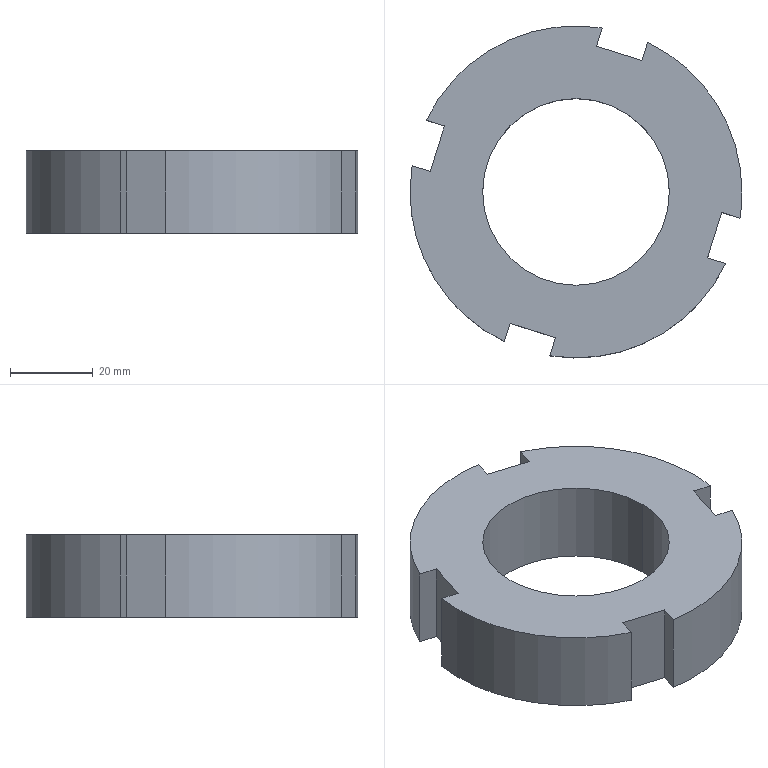Part | SolidWorks | features Extrusion 1 | 1 solid | 21 faces | box 80 x 80 x 20 mm | volume 64249 mm3 | plane 14 | cylinder 7 | commonest cylinder face diameters 80 x5 45 x2
STEP:
#1=CARTESIAN_POINT('',(498.731,234.744,-1569.998));
#2=VERTEX_POINT('',#1);
#3=CARTESIAN_POINT('',(543.731,234.744,-1569.998));
#4=VERTEX_POINT('',#3);
#5=CARTESIAN_POINT('',(521.231,234.744,-1569.998));
#6=DIRECTION('',(0.,0.,1.));
#7=DIRECTION('',(-1.,0.,0.));
#8=AXIS2_PLACEMENT_3D('',#5,#6,#7);
#9=CIRCLE('',#8,22.5);
#10=EDGE_CURVE('',#2,#4,#9,.T.);
#11=ORIENTED_EDGE('',*,*,#10,.F.);
#12=CARTESIAN_POINT('',(498.731,234.744,-1549.998));
#13=VERTEX_POINT('',#12);
#14=CARTESIAN_POINT('',(498.731,234.744,-1569.998));
#15=DIRECTION('',(0.,0.,1.));
#16=VECTOR('',#15,1000.);
#17=LINE('',#14,#16);
#18=EDGE_CURVE('',#2,#13,#17,.T.);
#19=ORIENTED_EDGE('',*,*,#18,.T.);
#20=CARTESIAN_POINT('',(543.731,234.744,-1549.998));
#21=VERTEX_POINT('',#20);
#22=CARTESIAN_POINT('',(521.231,234.744,-1549.998));
#23=DIRECTION('',(0.,0.,1.));
#24=DIRECTION('',(-1.,0.,0.));
#25=AXIS2_PLACEMENT_3D('',#22,#23,#24);
#26=CIRCLE('',#25,22.5);
#27=EDGE_CURVE('',#13,#21,#26,.T.);
#28=ORIENTED_EDGE('',*,*,#27,.T.);
#29=CARTESIAN_POINT('',(543.731,234.744,-1569.998));
#30=DIRECTION('',(0.,0.,1.));
#31=VECTOR('',#30,1000.);
#32=LINE('',#29,#31);
#33=EDGE_CURVE('',#4,#21,#32,.T.);
#34=ORIENTED_EDGE('',*,*,#33,.F.);
#35=EDGE_LOOP('',(#11,#19,#28,#34));
#36=FACE_OUTER_BOUND('',#35,.T.);
#37=CARTESIAN_POINT('',(521.231,234.744,-1569.998));
#38=DIRECTION('',(0.,0.,1.));
#39=DIRECTION('',(1.,0.,0.));
#40=AXIS2_PLACEMENT_3D('',#37,#38,#39);
#41=CYLINDRICAL_SURFACE('',#40,22.5);
#42=ADVANCED_FACE('',(#36),#41,.F.);
#43=CARTESIAN_POINT('',(560.733,228.457,-1569.998));
#44=VERTEX_POINT('',#43);
#45=CARTESIAN_POINT('',(561.231,234.744,-1569.998));
#46=VERTEX_POINT('',#45);
#47=CARTESIAN_POINT('',(521.231,234.744,-1569.998));
#48=DIRECTION('',(0.,0.,1.));
#49=DIRECTION('',(1.,0.,0.));
#50=AXIS2_PLACEMENT_3D('',#47,#48,#49);
#51=CIRCLE('',#50,40.);
#52=EDGE_CURVE('',#44,#46,#51,.T.);
#53=ORIENTED_EDGE('',*,*,#52,.T.);
#54=CARTESIAN_POINT('',(561.231,234.744,-1549.998));
#55=VERTEX_POINT('',#54);
#56=CARTESIAN_POINT('',(561.231,234.744,-1569.998));
#57=DIRECTION('',(0.,0.,1.));
#58=VECTOR('',#57,1000.);
#59=LINE('',#56,#58);
#60=EDGE_CURVE('',#46,#55,#59,.T.);
#61=ORIENTED_EDGE('',*,*,#60,.T.);
#62=CARTESIAN_POINT('',(560.733,228.457,-1549.998));
#63=VERTEX_POINT('',#62);
#64=CARTESIAN_POINT('',(521.231,234.744,-1549.998));
#65=DIRECTION('',(0.,0.,1.));
#66=DIRECTION('',(1.,0.,0.));
#67=AXIS2_PLACEMENT_3D('',#64,#65,#66);
#68=CIRCLE('',#67,40.);
#69=EDGE_CURVE('',#63,#55,#68,.T.);
#70=ORIENTED_EDGE('',*,*,#69,.F.);
#71=CARTESIAN_POINT('',(560.733,228.457,-1569.998));
#72=DIRECTION('',(0.,0.,1.));
#73=VECTOR('',#72,1000.);
#74=LINE('',#71,#73);
#75=EDGE_CURVE('',#44,#63,#74,.T.);
#76=ORIENTED_EDGE('',*,*,#75,.F.);
#77=EDGE_LOOP('',(#53,#61,#70,#76));
#78=FACE_OUTER_BOUND('',#77,.T.);
#79=CARTESIAN_POINT('',(521.231,234.744,-1569.998));
#80=DIRECTION('',(0.,0.,1.));
#81=DIRECTION('',(1.,0.,0.));
#82=AXIS2_PLACEMENT_3D('',#79,#80,#81);
#83=CYLINDRICAL_SURFACE('',#82,40.);
#84=ADVANCED_FACE('',(#78),#83,.T.);
#85=CARTESIAN_POINT('',(537.133,266.448,-1549.998));
#86=VERTEX_POINT('',#85);
#87=CARTESIAN_POINT('',(526.154,269.87,-1549.998));
#88=VERTEX_POINT('',#87);
#89=CARTESIAN_POINT('',(537.133,266.448,-1549.998));
#90=DIRECTION('',(-0.9547,0.2975,0.));
#91=VECTOR('',#90,1000.);
#92=LINE('',#89,#91);
#93=EDGE_CURVE('',#86,#88,#92,.T.);
#94=ORIENTED_EDGE('',*,*,#93,.F.);
#95=CARTESIAN_POINT('',(537.133,266.448,-1569.998));
#96=VERTEX_POINT('',#95);
#97=CARTESIAN_POINT('',(537.133,266.448,-1569.998));
#98=DIRECTION('',(0.,0.,1.));
#99=VECTOR('',#98,1000.);
#100=LINE('',#97,#99);
#101=EDGE_CURVE('',#96,#86,#100,.T.);
#102=ORIENTED_EDGE('',*,*,#101,.F.);
#103=CARTESIAN_POINT('',(526.154,269.87,-1569.998));
#104=VERTEX_POINT('',#103);
#105=CARTESIAN_POINT('',(537.133,266.448,-1569.998));
#106=DIRECTION('',(-0.9547,0.2975,0.));
#107=VECTOR('',#106,1000.);
#108=LINE('',#105,#107);
#109=EDGE_CURVE('',#96,#104,#108,.T.);
#110=ORIENTED_EDGE('',*,*,#109,.T.);
#111=CARTESIAN_POINT('',(526.154,269.87,-1569.998));
#112=DIRECTION('',(0.,0.,1.));
#113=VECTOR('',#112,1000.);
#114=LINE('',#111,#113);
#115=EDGE_CURVE('',#104,#88,#114,.T.);
#116=ORIENTED_EDGE('',*,*,#115,.T.);
#117=EDGE_LOOP('',(#94,#102,#110,#116));
#118=FACE_OUTER_BOUND('',#117,.T.);
#119=CARTESIAN_POINT('',(537.133,266.448,-1569.998));
#120=DIRECTION('',(0.2975,0.9547,0.));
#121=DIRECTION('',(-0.9547,0.2975,0.));
#122=AXIS2_PLACEMENT_3D('',#119,#120,#121);
#123=PLANE('',#122);
#124=ADVANCED_FACE('',(#118),#123,.T.);
#125=CARTESIAN_POINT('',(538.497,270.825,-1549.998));
#126=VERTEX_POINT('',#125);
#127=CARTESIAN_POINT('',(538.497,270.825,-1549.998));
#128=DIRECTION('',(-0.2975,-0.9547,0.));
#129=VECTOR('',#128,1000.);
#130=LINE('',#127,#129);
#131=EDGE_CURVE('',#126,#86,#130,.T.);
#132=ORIENTED_EDGE('',*,*,#131,.F.);
#133=CARTESIAN_POINT('',(538.497,270.825,-1569.998));
#134=VERTEX_POINT('',#133);
#135=CARTESIAN_POINT('',(538.497,270.825,-1569.998));
#136=DIRECTION('',(0.,0.,1.));
#137=VECTOR('',#136,1000.);
#138=LINE('',#135,#137);
#139=EDGE_CURVE('',#134,#126,#138,.T.);
#140=ORIENTED_EDGE('',*,*,#139,.F.);
#141=CARTESIAN_POINT('',(538.497,270.825,-1569.998));
#142=DIRECTION('',(-0.2975,-0.9547,0.));
#143=VECTOR('',#142,1000.);
#144=LINE('',#141,#143);
#145=EDGE_CURVE('',#134,#96,#144,.T.);
#146=ORIENTED_EDGE('',*,*,#145,.T.);
#147=ORIENTED_EDGE('',*,*,#101,.T.);
#148=EDGE_LOOP('',(#132,#140,#146,#147));
#149=FACE_OUTER_BOUND('',#148,.T.);
#150=CARTESIAN_POINT('',(538.497,270.825,-1569.998));
#151=DIRECTION('',(-0.9547,0.2975,0.));
#152=DIRECTION('',(-0.2975,-0.9547,0.));
#153=AXIS2_PLACEMENT_3D('',#150,#151,#152);
#154=PLANE('',#153);
#155=ADVANCED_FACE('',(#149),#154,.T.);
#156=ORIENTED_EDGE('',*,*,#60,.F.);
#157=CARTESIAN_POINT('',(521.231,234.744,-1569.998));
#158=DIRECTION('',(0.,0.,1.));
#159=DIRECTION('',(1.,0.,0.));
#160=AXIS2_PLACEMENT_3D('',#157,#158,#159);
#161=CIRCLE('',#160,40.);
#162=EDGE_CURVE('',#46,#134,#161,.T.);
#163=ORIENTED_EDGE('',*,*,#162,.T.);
#164=ORIENTED_EDGE('',*,*,#139,.T.);
#165=CARTESIAN_POINT('',(521.231,234.744,-1549.998));
#166=DIRECTION('',(0.,0.,1.));
#167=DIRECTION('',(1.,0.,0.));
#168=AXIS2_PLACEMENT_3D('',#165,#166,#167);
#169=CIRCLE('',#168,40.);
#170=EDGE_CURVE('',#55,#126,#169,.T.);
#171=ORIENTED_EDGE('',*,*,#170,.F.);
#172=EDGE_LOOP('',(#156,#163,#164,#171));
#173=FACE_OUTER_BOUND('',#172,.T.);
#174=CARTESIAN_POINT('',(521.231,234.744,-1569.998));
#175=DIRECTION('',(0.,0.,1.));
#176=DIRECTION('',(1.,0.,0.));
#177=AXIS2_PLACEMENT_3D('',#174,#175,#176);
#178=CYLINDRICAL_SURFACE('',#177,40.);
#179=ADVANCED_FACE('',(#173),#178,.T.);
#180=CARTESIAN_POINT('',(556.356,229.821,-1549.998));
#181=VERTEX_POINT('',#180);
#182=CARTESIAN_POINT('',(556.356,229.821,-1549.998));
#183=DIRECTION('',(0.9547,-0.2975,0.));
#184=VECTOR('',#183,1000.);
#185=LINE('',#182,#184);
#186=EDGE_CURVE('',#181,#63,#185,.T.);
#187=ORIENTED_EDGE('',*,*,#186,.F.);
#188=CARTESIAN_POINT('',(556.356,229.821,-1569.998));
#189=VERTEX_POINT('',#188);
#190=CARTESIAN_POINT('',(556.356,229.821,-1569.998));
#191=DIRECTION('',(0.,0.,1.));
#192=VECTOR('',#191,1000.);
#193=LINE('',#190,#192);
#194=EDGE_CURVE('',#189,#181,#193,.T.);
#195=ORIENTED_EDGE('',*,*,#194,.F.);
#196=CARTESIAN_POINT('',(556.356,229.821,-1569.998));
#197=DIRECTION('',(0.9547,-0.2975,0.));
#198=VECTOR('',#197,1000.);
#199=LINE('',#196,#198);
#200=EDGE_CURVE('',#189,#44,#199,.T.);
#201=ORIENTED_EDGE('',*,*,#200,.T.);
#202=ORIENTED_EDGE('',*,*,#75,.T.);
#203=EDGE_LOOP('',(#187,#195,#201,#202));
#204=FACE_OUTER_BOUND('',#203,.T.);
#205=CARTESIAN_POINT('',(556.356,229.821,-1569.998));
#206=DIRECTION('',(-0.2975,-0.9547,0.));
#207=DIRECTION('',(0.9547,-0.2975,0.));
#208=AXIS2_PLACEMENT_3D('',#205,#206,#207);
#209=PLANE('',#208);
#210=ADVANCED_FACE('',(#204),#209,.T.);
#211=CARTESIAN_POINT('',(552.935,218.841,-1549.998));
#212=VERTEX_POINT('',#211);
#213=CARTESIAN_POINT('',(552.935,218.841,-1549.998));
#214=DIRECTION('',(0.2975,0.9547,0.));
#215=VECTOR('',#214,1000.);
#216=LINE('',#213,#215);
#217=EDGE_CURVE('',#212,#181,#216,.T.);
#218=ORIENTED_EDGE('',*,*,#217,.F.);
#219=CARTESIAN_POINT('',(552.935,218.841,-1569.998));
#220=VERTEX_POINT('',#219);
#221=CARTESIAN_POINT('',(552.935,218.841,-1569.998));
#222=DIRECTION('',(0.,0.,1.));
#223=VECTOR('',#222,1000.);
#224=LINE('',#221,#223);
#225=EDGE_CURVE('',#220,#212,#224,.T.);
#226=ORIENTED_EDGE('',*,*,#225,.F.);
#227=CARTESIAN_POINT('',(552.935,218.841,-1569.998));
#228=DIRECTION('',(0.2975,0.9547,0.));
#229=VECTOR('',#228,1000.);
#230=LINE('',#227,#229);
#231=EDGE_CURVE('',#220,#189,#230,.T.);
#232=ORIENTED_EDGE('',*,*,#231,.T.);
#233=ORIENTED_EDGE('',*,*,#194,.T.);
#234=EDGE_LOOP('',(#218,#226,#232,#233));
#235=FACE_OUTER_BOUND('',#234,.T.);
#236=CARTESIAN_POINT('',(552.935,218.841,-1569.998));
#237=DIRECTION('',(0.9547,-0.2975,0.));
#238=DIRECTION('',(0.2975,0.9547,0.));
#239=AXIS2_PLACEMENT_3D('',#236,#237,#238);
#240=PLANE('',#239);
#241=ADVANCED_FACE('',(#235),#240,.T.);
#242=CARTESIAN_POINT('',(557.312,217.477,-1549.998));
#243=VERTEX_POINT('',#242);
#244=CARTESIAN_POINT('',(557.312,217.477,-1549.998));
#245=DIRECTION('',(-0.9547,0.2975,0.));
#246=VECTOR('',#245,1000.);
#247=LINE('',#244,#246);
#248=EDGE_CURVE('',#243,#212,#247,.T.);
#249=ORIENTED_EDGE('',*,*,#248,.F.);
#250=CARTESIAN_POINT('',(557.312,217.477,-1569.998));
#251=VERTEX_POINT('',#250);
#252=CARTESIAN_POINT('',(557.312,217.477,-1569.998));
#253=DIRECTION('',(0.,0.,1.));
#254=VECTOR('',#253,1000.);
#255=LINE('',#252,#254);
#256=EDGE_CURVE('',#251,#243,#255,.T.);
#257=ORIENTED_EDGE('',*,*,#256,.F.);
#258=CARTESIAN_POINT('',(557.312,217.477,-1569.998));
#259=DIRECTION('',(-0.9547,0.2975,0.));
#260=VECTOR('',#259,1000.);
#261=LINE('',#258,#260);
#262=EDGE_CURVE('',#251,#220,#261,.T.);
#263=ORIENTED_EDGE('',*,*,#262,.T.);
#264=ORIENTED_EDGE('',*,*,#225,.T.);
#265=EDGE_LOOP('',(#249,#257,#263,#264));
#266=FACE_OUTER_BOUND('',#265,.T.);
#267=CARTESIAN_POINT('',(557.312,217.477,-1569.998));
#268=DIRECTION('',(0.2975,0.9547,0.));
#269=DIRECTION('',(-0.9547,0.2975,0.));
#270=AXIS2_PLACEMENT_3D('',#267,#268,#269);
#271=PLANE('',#270);
#272=ADVANCED_FACE('',(#266),#271,.T.);
#273=CARTESIAN_POINT('',(514.943,195.241,-1549.998));
#274=VERTEX_POINT('',#273);
#275=CARTESIAN_POINT('',(521.231,234.744,-1549.998));
#276=DIRECTION('',(0.,0.,1.));
#277=DIRECTION('',(1.,0.,0.));
#278=AXIS2_PLACEMENT_3D('',#275,#276,#277);
#279=CIRCLE('',#278,40.);
#280=EDGE_CURVE('',#274,#243,#279,.T.);
#281=ORIENTED_EDGE('',*,*,#280,.F.);
#282=CARTESIAN_POINT('',(514.943,195.241,-1569.998));
#283=VERTEX_POINT('',#282);
#284=CARTESIAN_POINT('',(514.943,195.241,-1569.998));
#285=DIRECTION('',(0.,0.,1.));
#286=VECTOR('',#285,1000.);
#287=LINE('',#284,#286);
#288=EDGE_CURVE('',#283,#274,#287,.T.);
#289=ORIENTED_EDGE('',*,*,#288,.F.);
#290=CARTESIAN_POINT('',(521.231,234.744,-1569.998));
#291=DIRECTION('',(0.,0.,1.));
#292=DIRECTION('',(1.,0.,0.));
#293=AXIS2_PLACEMENT_3D('',#290,#291,#292);
#294=CIRCLE('',#293,40.);
#295=EDGE_CURVE('',#283,#251,#294,.T.);
#296=ORIENTED_EDGE('',*,*,#295,.T.);
#297=ORIENTED_EDGE('',*,*,#256,.T.);
#298=EDGE_LOOP('',(#281,#289,#296,#297));
#299=FACE_OUTER_BOUND('',#298,.T.);
#300=CARTESIAN_POINT('',(521.231,234.744,-1569.998));
#301=DIRECTION('',(0.,0.,1.));
#302=DIRECTION('',(1.,0.,0.));
#303=AXIS2_PLACEMENT_3D('',#300,#301,#302);
#304=CYLINDRICAL_SURFACE('',#303,40.);
#305=ADVANCED_FACE('',(#299),#304,.T.);
#306=CARTESIAN_POINT('',(516.307,199.618,-1549.998));
#307=VERTEX_POINT('',#306);
#308=CARTESIAN_POINT('',(516.307,199.618,-1549.998));
#309=DIRECTION('',(-0.2975,-0.9547,0.));
#310=VECTOR('',#309,1000.);
#311=LINE('',#308,#310);
#312=EDGE_CURVE('',#307,#274,#311,.T.);
#313=ORIENTED_EDGE('',*,*,#312,.F.);
#314=CARTESIAN_POINT('',(516.307,199.618,-1569.998));
#315=VERTEX_POINT('',#314);
#316=CARTESIAN_POINT('',(516.307,199.618,-1569.998));
#317=DIRECTION('',(0.,0.,1.));
#318=VECTOR('',#317,1000.);
#319=LINE('',#316,#318);
#320=EDGE_CURVE('',#315,#307,#319,.T.);
#321=ORIENTED_EDGE('',*,*,#320,.F.);
#322=CARTESIAN_POINT('',(516.307,199.618,-1569.998));
#323=DIRECTION('',(-0.2975,-0.9547,0.));
#324=VECTOR('',#323,1000.);
#325=LINE('',#322,#324);
#326=EDGE_CURVE('',#315,#283,#325,.T.);
#327=ORIENTED_EDGE('',*,*,#326,.T.);
#328=ORIENTED_EDGE('',*,*,#288,.T.);
#329=EDGE_LOOP('',(#313,#321,#327,#328));
#330=FACE_OUTER_BOUND('',#329,.T.);
#331=CARTESIAN_POINT('',(516.307,199.618,-1569.998));
#332=DIRECTION('',(-0.9547,0.2975,0.));
#333=DIRECTION('',(-0.2975,-0.9547,0.));
#334=AXIS2_PLACEMENT_3D('',#331,#332,#333);
#335=PLANE('',#334);
#336=ADVANCED_FACE('',(#330),#335,.T.);
#337=CARTESIAN_POINT('',(505.328,203.04,-1549.998));
#338=VERTEX_POINT('',#337);
#339=CARTESIAN_POINT('',(505.328,203.04,-1549.998));
#340=DIRECTION('',(0.9547,-0.2975,0.));
#341=VECTOR('',#340,1000.);
#342=LINE('',#339,#341);
#343=EDGE_CURVE('',#338,#307,#342,.T.);
#344=ORIENTED_EDGE('',*,*,#343,.F.);
#345=CARTESIAN_POINT('',(505.328,203.04,-1569.998));
#346=VERTEX_POINT('',#345);
#347=CARTESIAN_POINT('',(505.328,203.04,-1569.998));
#348=DIRECTION('',(0.,0.,1.));
#349=VECTOR('',#348,1000.);
#350=LINE('',#347,#349);
#351=EDGE_CURVE('',#346,#338,#350,.T.);
#352=ORIENTED_EDGE('',*,*,#351,.F.);
#353=CARTESIAN_POINT('',(505.328,203.04,-1569.998));
#354=DIRECTION('',(0.9547,-0.2975,0.));
#355=VECTOR('',#354,1000.);
#356=LINE('',#353,#355);
#357=EDGE_CURVE('',#346,#315,#356,.T.);
#358=ORIENTED_EDGE('',*,*,#357,.T.);
#359=ORIENTED_EDGE('',*,*,#320,.T.);
#360=EDGE_LOOP('',(#344,#352,#358,#359));
#361=FACE_OUTER_BOUND('',#360,.T.);
#362=CARTESIAN_POINT('',(505.328,203.04,-1569.998));
#363=DIRECTION('',(-0.2975,-0.9547,0.));
#364=DIRECTION('',(0.9547,-0.2975,0.));
#365=AXIS2_PLACEMENT_3D('',#362,#363,#364);
#366=PLANE('',#365);
#367=ADVANCED_FACE('',(#361),#366,.T.);
#368=CARTESIAN_POINT('',(503.964,198.663,-1549.998));
#369=VERTEX_POINT('',#368);
#370=CARTESIAN_POINT('',(503.964,198.663,-1549.998));
#371=DIRECTION('',(0.2975,0.9547,0.));
#372=VECTOR('',#371,1000.);
#373=LINE('',#370,#372);
#374=EDGE_CURVE('',#369,#338,#373,.T.);
#375=ORIENTED_EDGE('',*,*,#374,.F.);
#376=CARTESIAN_POINT('',(503.964,198.663,-1569.998));
#377=VERTEX_POINT('',#376);
#378=CARTESIAN_POINT('',(503.964,198.663,-1569.998));
#379=DIRECTION('',(0.,0.,1.));
#380=VECTOR('',#379,1000.);
#381=LINE('',#378,#380);
#382=EDGE_CURVE('',#377,#369,#381,.T.);
#383=ORIENTED_EDGE('',*,*,#382,.F.);
#384=CARTESIAN_POINT('',(503.964,198.663,-1569.998));
#385=DIRECTION('',(0.2975,0.9547,0.));
#386=VECTOR('',#385,1000.);
#387=LINE('',#384,#386);
#388=EDGE_CURVE('',#377,#346,#387,.T.);
#389=ORIENTED_EDGE('',*,*,#388,.T.);
#390=ORIENTED_EDGE('',*,*,#351,.T.);
#391=EDGE_LOOP('',(#375,#383,#389,#390));
#392=FACE_OUTER_BOUND('',#391,.T.);
#393=CARTESIAN_POINT('',(503.964,198.663,-1569.998));
#394=DIRECTION('',(0.9547,-0.2975,0.));
#395=DIRECTION('',(0.2975,0.9547,0.));
#396=AXIS2_PLACEMENT_3D('',#393,#394,#395);
#397=PLANE('',#396);
#398=ADVANCED_FACE('',(#392),#397,.T.);
#399=CARTESIAN_POINT('',(481.728,241.031,-1549.998));
#400=VERTEX_POINT('',#399);
#401=CARTESIAN_POINT('',(521.231,234.744,-1549.998));
#402=DIRECTION('',(0.,0.,1.));
#403=DIRECTION('',(1.,0.,0.));
#404=AXIS2_PLACEMENT_3D('',#401,#402,#403);
#405=CIRCLE('',#404,40.);
#406=EDGE_CURVE('',#400,#369,#405,.T.);
#407=ORIENTED_EDGE('',*,*,#406,.F.);
#408=CARTESIAN_POINT('',(481.728,241.031,-1569.998));
#409=VERTEX_POINT('',#408);
#410=CARTESIAN_POINT('',(481.728,241.031,-1569.998));
#411=DIRECTION('',(0.,0.,1.));
#412=VECTOR('',#411,1000.);
#413=LINE('',#410,#412);
#414=EDGE_CURVE('',#409,#400,#413,.T.);
#415=ORIENTED_EDGE('',*,*,#414,.F.);
#416=CARTESIAN_POINT('',(521.231,234.744,-1569.998));
#417=DIRECTION('',(0.,0.,1.));
#418=DIRECTION('',(1.,0.,0.));
#419=AXIS2_PLACEMENT_3D('',#416,#417,#418);
#420=CIRCLE('',#419,40.);
#421=EDGE_CURVE('',#409,#377,#420,.T.);
#422=ORIENTED_EDGE('',*,*,#421,.T.);
#423=ORIENTED_EDGE('',*,*,#382,.T.);
#424=EDGE_LOOP('',(#407,#415,#422,#423));
#425=FACE_OUTER_BOUND('',#424,.T.);
#426=CARTESIAN_POINT('',(521.231,234.744,-1569.998));
#427=DIRECTION('',(0.,0.,1.));
#428=DIRECTION('',(1.,0.,0.));
#429=AXIS2_PLACEMENT_3D('',#426,#427,#428);
#430=CYLINDRICAL_SURFACE('',#429,40.);
#431=ADVANCED_FACE('',(#425),#430,.T.);
#432=CARTESIAN_POINT('',(486.105,239.667,-1549.998));
#433=VERTEX_POINT('',#432);
#434=CARTESIAN_POINT('',(486.105,239.667,-1549.998));
#435=DIRECTION('',(-0.9547,0.2975,0.));
#436=VECTOR('',#435,1000.);
#437=LINE('',#434,#436);
#438=EDGE_CURVE('',#433,#400,#437,.T.);
#439=ORIENTED_EDGE('',*,*,#438,.F.);
#440=CARTESIAN_POINT('',(486.105,239.667,-1569.998));
#441=VERTEX_POINT('',#440);
#442=CARTESIAN_POINT('',(486.105,239.667,-1569.998));
#443=DIRECTION('',(0.,0.,1.));
#444=VECTOR('',#443,1000.);
#445=LINE('',#442,#444);
#446=EDGE_CURVE('',#441,#433,#445,.T.);
#447=ORIENTED_EDGE('',*,*,#446,.F.);
#448=CARTESIAN_POINT('',(486.105,239.667,-1569.998));
#449=DIRECTION('',(-0.9547,0.2975,0.));
#450=VECTOR('',#449,1000.);
#451=LINE('',#448,#450);
#452=EDGE_CURVE('',#441,#409,#451,.T.);
#453=ORIENTED_EDGE('',*,*,#452,.T.);
#454=ORIENTED_EDGE('',*,*,#414,.T.);
#455=EDGE_LOOP('',(#439,#447,#453,#454));
#456=FACE_OUTER_BOUND('',#455,.T.);
#457=CARTESIAN_POINT('',(486.105,239.667,-1569.998));
#458=DIRECTION('',(0.2975,0.9547,0.));
#459=DIRECTION('',(-0.9547,0.2975,0.));
#460=AXIS2_PLACEMENT_3D('',#457,#458,#459);
#461=PLANE('',#460);
#462=ADVANCED_FACE('',(#456),#461,.T.);
#463=CARTESIAN_POINT('',(489.526,250.647,-1549.998));
#464=VERTEX_POINT('',#463);
#465=CARTESIAN_POINT('',(489.526,250.647,-1549.998));
#466=DIRECTION('',(-0.2975,-0.9547,0.));
#467=VECTOR('',#466,1000.);
#468=LINE('',#465,#467);
#469=EDGE_CURVE('',#464,#433,#468,.T.);
#470=ORIENTED_EDGE('',*,*,#469,.F.);
#471=CARTESIAN_POINT('',(489.526,250.647,-1569.998));
#472=VERTEX_POINT('',#471);
#473=CARTESIAN_POINT('',(489.526,250.647,-1569.998));
#474=DIRECTION('',(0.,0.,1.));
#475=VECTOR('',#474,1000.);
#476=LINE('',#473,#475);
#477=EDGE_CURVE('',#472,#464,#476,.T.);
#478=ORIENTED_EDGE('',*,*,#477,.F.);
#479=CARTESIAN_POINT('',(489.526,250.647,-1569.998));
#480=DIRECTION('',(-0.2975,-0.9547,0.));
#481=VECTOR('',#480,1000.);
#482=LINE('',#479,#481);
#483=EDGE_CURVE('',#472,#441,#482,.T.);
#484=ORIENTED_EDGE('',*,*,#483,.T.);
#485=ORIENTED_EDGE('',*,*,#446,.T.);
#486=EDGE_LOOP('',(#470,#478,#484,#485));
#487=FACE_OUTER_BOUND('',#486,.T.);
#488=CARTESIAN_POINT('',(489.526,250.647,-1569.998));
#489=DIRECTION('',(-0.9547,0.2975,0.));
#490=DIRECTION('',(-0.2975,-0.9547,0.));
#491=AXIS2_PLACEMENT_3D('',#488,#489,#490);
#492=PLANE('',#491);
#493=ADVANCED_FACE('',(#487),#492,.T.);
#494=CARTESIAN_POINT('',(485.149,252.011,-1549.998));
#495=VERTEX_POINT('',#494);
#496=CARTESIAN_POINT('',(485.149,252.011,-1549.998));
#497=DIRECTION('',(0.9547,-0.2975,0.));
#498=VECTOR('',#497,1000.);
#499=LINE('',#496,#498);
#500=EDGE_CURVE('',#495,#464,#499,.T.);
#501=ORIENTED_EDGE('',*,*,#500,.F.);
#502=CARTESIAN_POINT('',(485.149,252.011,-1569.998));
#503=VERTEX_POINT('',#502);
#504=CARTESIAN_POINT('',(485.149,252.011,-1569.998));
#505=DIRECTION('',(0.,0.,1.));
#506=VECTOR('',#505,1000.);
#507=LINE('',#504,#506);
#508=EDGE_CURVE('',#503,#495,#507,.T.);
#509=ORIENTED_EDGE('',*,*,#508,.F.);
#510=CARTESIAN_POINT('',(485.149,252.011,-1569.998));
#511=DIRECTION('',(0.9547,-0.2975,0.));
#512=VECTOR('',#511,1000.);
#513=LINE('',#510,#512);
#514=EDGE_CURVE('',#503,#472,#513,.T.);
#515=ORIENTED_EDGE('',*,*,#514,.T.);
#516=ORIENTED_EDGE('',*,*,#477,.T.);
#517=EDGE_LOOP('',(#501,#509,#515,#516));
#518=FACE_OUTER_BOUND('',#517,.T.);
#519=CARTESIAN_POINT('',(485.149,252.011,-1569.998));
#520=DIRECTION('',(-0.2975,-0.9547,0.));
#521=DIRECTION('',(0.9547,-0.2975,0.));
#522=AXIS2_PLACEMENT_3D('',#519,#520,#521);
#523=PLANE('',#522);
#524=ADVANCED_FACE('',(#518),#523,.T.);
#525=CARTESIAN_POINT('',(527.518,274.247,-1549.998));
#526=VERTEX_POINT('',#525);
#527=CARTESIAN_POINT('',(521.231,234.744,-1549.998));
#528=DIRECTION('',(0.,0.,1.));
#529=DIRECTION('',(1.,0.,0.));
#530=AXIS2_PLACEMENT_3D('',#527,#528,#529);
#531=CIRCLE('',#530,40.);
#532=EDGE_CURVE('',#526,#495,#531,.T.);
#533=ORIENTED_EDGE('',*,*,#532,.F.);
#534=CARTESIAN_POINT('',(527.518,274.247,-1569.998));
#535=VERTEX_POINT('',#534);
#536=CARTESIAN_POINT('',(527.518,274.247,-1569.998));
#537=DIRECTION('',(0.,0.,1.));
#538=VECTOR('',#537,1000.);
#539=LINE('',#536,#538);
#540=EDGE_CURVE('',#535,#526,#539,.T.);
#541=ORIENTED_EDGE('',*,*,#540,.F.);
#542=CARTESIAN_POINT('',(521.231,234.744,-1569.998));
#543=DIRECTION('',(0.,0.,1.));
#544=DIRECTION('',(1.,0.,0.));
#545=AXIS2_PLACEMENT_3D('',#542,#543,#544);
#546=CIRCLE('',#545,40.);
#547=EDGE_CURVE('',#535,#503,#546,.T.);
#548=ORIENTED_EDGE('',*,*,#547,.T.);
#549=ORIENTED_EDGE('',*,*,#508,.T.);
#550=EDGE_LOOP('',(#533,#541,#548,#549));
#551=FACE_OUTER_BOUND('',#550,.T.);
#552=CARTESIAN_POINT('',(521.231,234.744,-1569.998));
#553=DIRECTION('',(0.,0.,1.));
#554=DIRECTION('',(1.,0.,0.));
#555=AXIS2_PLACEMENT_3D('',#552,#553,#554);
#556=CYLINDRICAL_SURFACE('',#555,40.);
#557=ADVANCED_FACE('',(#551),#556,.T.);
#558=CARTESIAN_POINT('',(526.154,269.87,-1549.998));
#559=DIRECTION('',(0.2975,0.9547,0.));
#560=VECTOR('',#559,1000.);
#561=LINE('',#558,#560);
#562=EDGE_CURVE('',#88,#526,#561,.T.);
#563=ORIENTED_EDGE('',*,*,#562,.F.);
#564=ORIENTED_EDGE('',*,*,#115,.F.);
#565=CARTESIAN_POINT('',(526.154,269.87,-1569.998));
#566=DIRECTION('',(0.2975,0.9547,0.));
#567=VECTOR('',#566,1000.);
#568=LINE('',#565,#567);
#569=EDGE_CURVE('',#104,#535,#568,.T.);
#570=ORIENTED_EDGE('',*,*,#569,.T.);
#571=ORIENTED_EDGE('',*,*,#540,.T.);
#572=EDGE_LOOP('',(#563,#564,#570,#571));
#573=FACE_OUTER_BOUND('',#572,.T.);
#574=CARTESIAN_POINT('',(526.154,269.87,-1569.998));
#575=DIRECTION('',(0.9547,-0.2975,0.));
#576=DIRECTION('',(0.2975,0.9547,0.));
#577=AXIS2_PLACEMENT_3D('',#574,#575,#576);
#578=PLANE('',#577);
#579=ADVANCED_FACE('',(#573),#578,.T.);
#580=CARTESIAN_POINT('',(521.231,234.744,-1569.998));
#581=DIRECTION('',(0.,0.,1.));
#582=DIRECTION('',(-1.,0.,0.));
#583=AXIS2_PLACEMENT_3D('',#580,#581,#582);
#584=CIRCLE('',#583,22.5);
#585=EDGE_CURVE('',#4,#2,#584,.T.);
#586=ORIENTED_EDGE('',*,*,#585,.T.);
#587=ORIENTED_EDGE('',*,*,#10,.T.);
#588=EDGE_LOOP('',(#586,#587));
#589=FACE_BOUND('',#588,.T.);
#590=ORIENTED_EDGE('',*,*,#109,.F.);
#591=ORIENTED_EDGE('',*,*,#145,.F.);
#592=ORIENTED_EDGE('',*,*,#162,.F.);
#593=ORIENTED_EDGE('',*,*,#52,.F.);
#594=ORIENTED_EDGE('',*,*,#200,.F.);
#595=ORIENTED_EDGE('',*,*,#231,.F.);
#596=ORIENTED_EDGE('',*,*,#262,.F.);
#597=ORIENTED_EDGE('',*,*,#295,.F.);
#598=ORIENTED_EDGE('',*,*,#326,.F.);
#599=ORIENTED_EDGE('',*,*,#357,.F.);
#600=ORIENTED_EDGE('',*,*,#388,.F.);
#601=ORIENTED_EDGE('',*,*,#421,.F.);
#602=ORIENTED_EDGE('',*,*,#452,.F.);
#603=ORIENTED_EDGE('',*,*,#483,.F.);
#604=ORIENTED_EDGE('',*,*,#514,.F.);
#605=ORIENTED_EDGE('',*,*,#547,.F.);
#606=ORIENTED_EDGE('',*,*,#569,.F.);
#607=EDGE_LOOP('',(#590,#591,#592,#593,#594,#595,#596,#597,#598,#599,#600,#601,#602,#603,#604,#605,#606));
#608=FACE_OUTER_BOUND('',#607,.T.);
#609=CARTESIAN_POINT('',(521.231,234.744,-1569.998));
#610=DIRECTION('',(0.,0.,1.));
#611=DIRECTION('',(1.,0.,0.));
#612=AXIS2_PLACEMENT_3D('',#609,#610,#611);
#613=PLANE('',#612);
#614=ADVANCED_FACE('',(#589,#608),#613,.F.);
#615=CARTESIAN_POINT('',(521.231,234.744,-1549.998));
#616=DIRECTION('',(0.,0.,1.));
#617=DIRECTION('',(-1.,0.,0.));
#618=AXIS2_PLACEMENT_3D('',#615,#616,#617);
#619=CIRCLE('',#618,22.5);
#620=EDGE_CURVE('',#21,#13,#619,.T.);
#621=ORIENTED_EDGE('',*,*,#620,.F.);
#622=ORIENTED_EDGE('',*,*,#27,.F.);
#623=EDGE_LOOP('',(#621,#622));
#624=FACE_BOUND('',#623,.T.);
#625=ORIENTED_EDGE('',*,*,#93,.T.);
#626=ORIENTED_EDGE('',*,*,#562,.T.);
#627=ORIENTED_EDGE('',*,*,#532,.T.);
#628=ORIENTED_EDGE('',*,*,#500,.T.);
#629=ORIENTED_EDGE('',*,*,#469,.T.);
#630=ORIENTED_EDGE('',*,*,#438,.T.);
#631=ORIENTED_EDGE('',*,*,#406,.T.);
#632=ORIENTED_EDGE('',*,*,#374,.T.);
#633=ORIENTED_EDGE('',*,*,#343,.T.);
#634=ORIENTED_EDGE('',*,*,#312,.T.);
#635=ORIENTED_EDGE('',*,*,#280,.T.);
#636=ORIENTED_EDGE('',*,*,#248,.T.);
#637=ORIENTED_EDGE('',*,*,#217,.T.);
#638=ORIENTED_EDGE('',*,*,#186,.T.);
#639=ORIENTED_EDGE('',*,*,#69,.T.);
#640=ORIENTED_EDGE('',*,*,#170,.T.);
#641=ORIENTED_EDGE('',*,*,#131,.T.);
#642=EDGE_LOOP('',(#625,#626,#627,#628,#629,#630,#631,#632,#633,#634,#635,#636,#637,#638,#639,#640,#641));
#643=FACE_OUTER_BOUND('',#642,.T.);
#644=CARTESIAN_POINT('',(521.231,234.744,-1549.998));
#645=DIRECTION('',(0.,0.,1.));
#646=DIRECTION('',(1.,0.,0.));
#647=AXIS2_PLACEMENT_3D('',#644,#645,#646);
#648=PLANE('',#647);
#649=ADVANCED_FACE('',(#624,#643),#648,.T.);
#650=ORIENTED_EDGE('',*,*,#18,.F.);
#651=ORIENTED_EDGE('',*,*,#585,.F.);
#652=ORIENTED_EDGE('',*,*,#33,.T.);
#653=ORIENTED_EDGE('',*,*,#620,.T.);
#654=EDGE_LOOP('',(#650,#651,#652,#653));
#655=FACE_OUTER_BOUND('',#654,.T.);
#656=CARTESIAN_POINT('',(521.231,234.744,-1569.998));
#657=DIRECTION('',(0.,0.,1.));
#658=DIRECTION('',(1.,0.,0.));
#659=AXIS2_PLACEMENT_3D('',#656,#657,#658);
#660=CYLINDRICAL_SURFACE('',#659,22.5);
#661=ADVANCED_FACE('',(#655),#660,.F.);
#662=CLOSED_SHELL('',(#42,#84,#124,#155,#179,#210,#241,#272,#305,#336,#367,#398,#431,#462,#493,#524,#557,#579,#614,#649,#661));
#663=MANIFOLD_SOLID_BREP('',#662);
#664=CARTESIAN_POINT('',(0.,0.,0.));
#665=DIRECTION('',(0.,0.,1.));
#666=DIRECTION('',(1.,0.,0.));
#667=AXIS2_PLACEMENT_3D('',#664,#665,#666);
#668=(LENGTH_UNIT()NAMED_UNIT(*)SI_UNIT(.MILLI.,.METRE.));
#669=UNCERTAINTY_MEASURE_WITH_UNIT(LENGTH_MEASURE(0.00001),#668,'','');
#670=(NAMED_UNIT(*)PLANE_ANGLE_UNIT()SI_UNIT($,.RADIAN.));
#671=(NAMED_UNIT(*)SI_UNIT($,.STERADIAN.)SOLID_ANGLE_UNIT());
#672=(GEOMETRIC_REPRESENTATION_CONTEXT(3)GLOBAL_UNCERTAINTY_ASSIGNED_CONTEXT((#669))GLOBAL_UNIT_ASSIGNED_CONTEXT((#668,#670,#671))REPRESENTATION_CONTEXT('',''));
#673=ADVANCED_BREP_SHAPE_REPRESENTATION('',(#663,#667),#672);